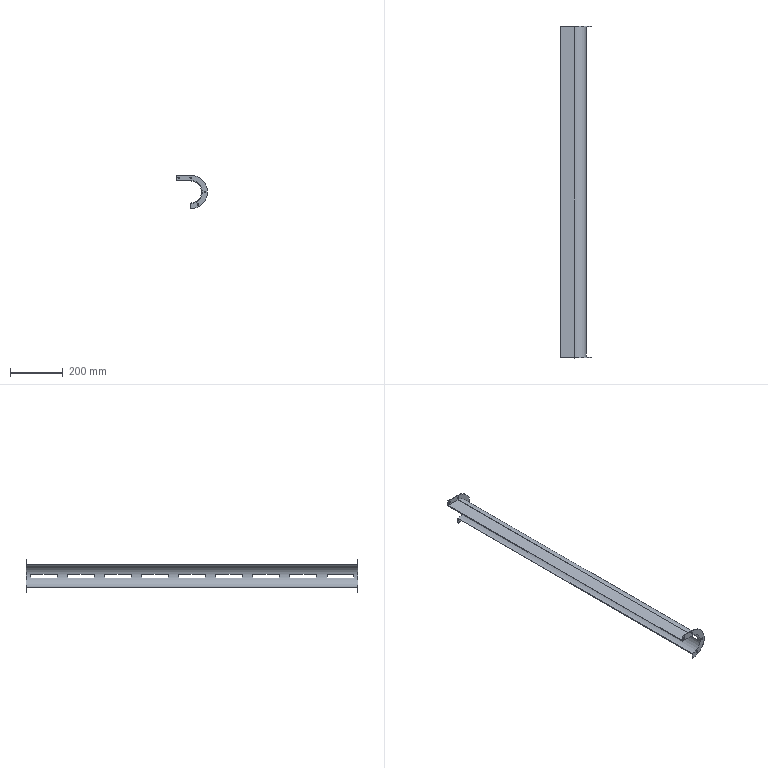Part | SolidWorks | features ICE 4, Extrusion 1 | 1 solid | 66 faces | box 117 x 1256 x 128 mm | volume 462770 mm3 | plane 46 | cylinder 20 | commonest cylinder face diameters 5.5 x16 128 x2 84 x1 88 x1